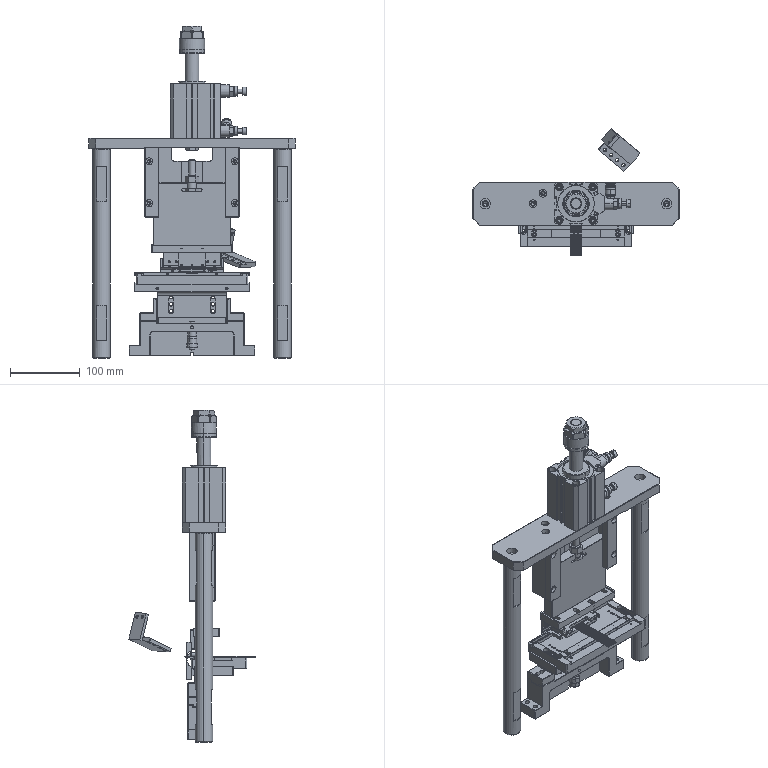Part | SolidWorks | 34 solids | 3008 faces | volume 1768279 mm3 | plane 1487 | cylinder 1102 | cone 296 | spline 107 | torus 12 | sphere 4 | commonest cylinder face diameters 0.1 x98 2.5 x90 0.4 x86 2 x67 0.16 x64 6.5 x58